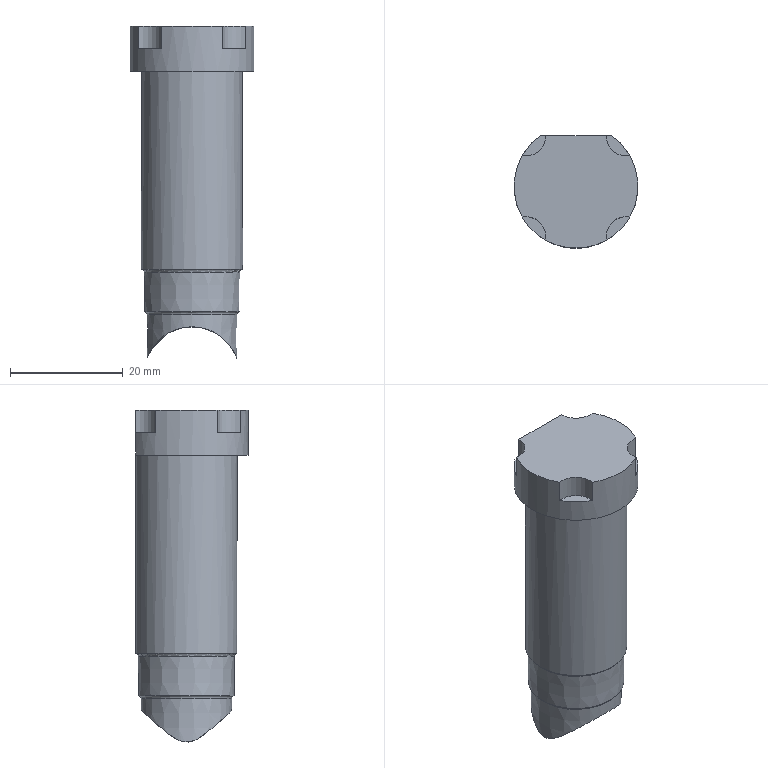Part | NX | features solid 2 | 1 solid | 18 faces | box 22 x 20 x 58.945 mm | volume 14202 mm3 | plane 7 | cylinder 6 | cone 3 | torus 2 | commonest cylinder face diameters 7 x4 18 x1 22 x1
STEP:
#1=CARTESIAN_POINT('',(9.556,23.036,66.5));
#2=VERTEX_POINT('',#1);
#3=CARTESIAN_POINT('',(6.325,26.587,66.5));
#4=VERTEX_POINT('',#3);
#5=CARTESIAN_POINT('',(0.,17.587,66.5));
#6=DIRECTION('',(0.,0.,-1.));
#7=DIRECTION('',(-1.,0.,0.));
#8=AXIS2_PLACEMENT_3D('',#5,#6,#7);
#9=CIRCLE('',#8,11.);
#10=EDGE_CURVE('',#2,#4,#9,.F.);
#11=ORIENTED_EDGE('',*,*,#10,.F.);
#12=CARTESIAN_POINT('',(9.556,23.036,70.5));
#13=VERTEX_POINT('',#12);
#14=CARTESIAN_POINT('',(9.556,23.036,66.5));
#15=DIRECTION('',(0.,0.,-1.));
#16=VECTOR('',#15,1000.);
#17=LINE('',#14,#16);
#18=EDGE_CURVE('',#2,#13,#17,.F.);
#19=ORIENTED_EDGE('',*,*,#18,.T.);
#20=CARTESIAN_POINT('',(9.556,12.139,70.5));
#21=VERTEX_POINT('',#20);
#22=CARTESIAN_POINT('',(0.,17.587,70.5));
#23=DIRECTION('',(0.,0.,1.));
#24=DIRECTION('',(1.,0.,0.));
#25=AXIS2_PLACEMENT_3D('',#22,#23,#24);
#26=CIRCLE('',#25,11.);
#27=EDGE_CURVE('',#21,#13,#26,.T.);
#28=ORIENTED_EDGE('',*,*,#27,.F.);
#29=CARTESIAN_POINT('',(9.556,12.139,66.5));
#30=VERTEX_POINT('',#29);
#31=CARTESIAN_POINT('',(9.556,12.139,66.5));
#32=DIRECTION('',(0.,0.,1.));
#33=VECTOR('',#32,1000.);
#34=LINE('',#31,#33);
#35=EDGE_CURVE('',#21,#30,#34,.F.);
#36=ORIENTED_EDGE('',*,*,#35,.T.);
#37=CARTESIAN_POINT('',(5.448,8.032,66.5));
#38=VERTEX_POINT('',#37);
#39=CARTESIAN_POINT('',(0.,17.587,66.5));
#40=DIRECTION('',(0.,0.,-1.));
#41=DIRECTION('',(-1.,0.,0.));
#42=AXIS2_PLACEMENT_3D('',#39,#40,#41);
#43=CIRCLE('',#42,11.);
#44=EDGE_CURVE('',#38,#30,#43,.F.);
#45=ORIENTED_EDGE('',*,*,#44,.F.);
#46=CARTESIAN_POINT('',(5.448,8.032,70.5));
#47=VERTEX_POINT('',#46);
#48=CARTESIAN_POINT('',(5.448,8.032,66.5));
#49=DIRECTION('',(0.,0.,1.));
#50=VECTOR('',#49,1000.);
#51=LINE('',#48,#50);
#52=EDGE_CURVE('',#38,#47,#51,.T.);
#53=ORIENTED_EDGE('',*,*,#52,.T.);
#54=CARTESIAN_POINT('',(-5.448,8.032,70.5));
#55=VERTEX_POINT('',#54);
#56=CARTESIAN_POINT('',(0.,17.587,70.5));
#57=DIRECTION('',(0.,0.,1.));
#58=DIRECTION('',(1.,0.,0.));
#59=AXIS2_PLACEMENT_3D('',#56,#57,#58);
#60=CIRCLE('',#59,11.);
#61=EDGE_CURVE('',#55,#47,#60,.T.);
#62=ORIENTED_EDGE('',*,*,#61,.F.);
#63=CARTESIAN_POINT('',(-5.448,8.032,66.5));
#64=VERTEX_POINT('',#63);
#65=CARTESIAN_POINT('',(-5.448,8.032,66.5));
#66=DIRECTION('',(0.,0.,1.));
#67=VECTOR('',#66,1000.);
#68=LINE('',#65,#67);
#69=EDGE_CURVE('',#55,#64,#68,.F.);
#70=ORIENTED_EDGE('',*,*,#69,.T.);
#71=CARTESIAN_POINT('',(-9.556,12.139,66.5));
#72=VERTEX_POINT('',#71);
#73=CARTESIAN_POINT('',(0.,17.587,66.5));
#74=DIRECTION('',(0.,0.,-1.));
#75=DIRECTION('',(-1.,0.,0.));
#76=AXIS2_PLACEMENT_3D('',#73,#74,#75);
#77=CIRCLE('',#76,11.);
#78=EDGE_CURVE('',#72,#64,#77,.F.);
#79=ORIENTED_EDGE('',*,*,#78,.F.);
#80=CARTESIAN_POINT('',(-9.556,12.139,70.5));
#81=VERTEX_POINT('',#80);
#82=CARTESIAN_POINT('',(-9.556,12.139,66.5));
#83=DIRECTION('',(0.,0.,1.));
#84=VECTOR('',#83,1000.);
#85=LINE('',#82,#84);
#86=EDGE_CURVE('',#72,#81,#85,.T.);
#87=ORIENTED_EDGE('',*,*,#86,.T.);
#88=CARTESIAN_POINT('',(-9.556,23.036,70.5));
#89=VERTEX_POINT('',#88);
#90=CARTESIAN_POINT('',(0.,17.587,70.5));
#91=DIRECTION('',(0.,0.,1.));
#92=DIRECTION('',(1.,0.,0.));
#93=AXIS2_PLACEMENT_3D('',#90,#91,#92);
#94=CIRCLE('',#93,11.);
#95=EDGE_CURVE('',#89,#81,#94,.T.);
#96=ORIENTED_EDGE('',*,*,#95,.F.);
#97=CARTESIAN_POINT('',(-9.556,23.036,66.5));
#98=VERTEX_POINT('',#97);
#99=CARTESIAN_POINT('',(-9.556,23.036,66.5));
#100=DIRECTION('',(0.,0.,1.));
#101=VECTOR('',#100,1000.);
#102=LINE('',#99,#101);
#103=EDGE_CURVE('',#89,#98,#102,.F.);
#104=ORIENTED_EDGE('',*,*,#103,.T.);
#105=CARTESIAN_POINT('',(-6.325,26.587,66.5));
#106=VERTEX_POINT('',#105);
#107=CARTESIAN_POINT('',(0.,17.587,66.5));
#108=DIRECTION('',(0.,0.,-1.));
#109=DIRECTION('',(-1.,0.,0.));
#110=AXIS2_PLACEMENT_3D('',#107,#108,#109);
#111=CIRCLE('',#110,11.);
#112=EDGE_CURVE('',#106,#98,#111,.F.);
#113=ORIENTED_EDGE('',*,*,#112,.F.);
#114=CARTESIAN_POINT('',(-6.325,26.587,62.5));
#115=VERTEX_POINT('',#114);
#116=CARTESIAN_POINT('',(-6.325,26.587,62.5));
#117=DIRECTION('',(0.,0.,1.));
#118=VECTOR('',#117,1000.);
#119=LINE('',#116,#118);
#120=EDGE_CURVE('',#106,#115,#119,.F.);
#121=ORIENTED_EDGE('',*,*,#120,.T.);
#122=CARTESIAN_POINT('',(6.325,26.587,62.5));
#123=VERTEX_POINT('',#122);
#124=CARTESIAN_POINT('',(0.,17.587,62.5));
#125=DIRECTION('',(0.,0.,1.));
#126=DIRECTION('',(1.,0.,0.));
#127=AXIS2_PLACEMENT_3D('',#124,#125,#126);
#128=CIRCLE('',#127,11.);
#129=EDGE_CURVE('',#115,#123,#128,.T.);
#130=ORIENTED_EDGE('',*,*,#129,.T.);
#131=CARTESIAN_POINT('',(6.325,26.587,62.5));
#132=DIRECTION('',(0.,0.,1.));
#133=VECTOR('',#132,1000.);
#134=LINE('',#131,#133);
#135=EDGE_CURVE('',#123,#4,#134,.T.);
#136=ORIENTED_EDGE('',*,*,#135,.T.);
#137=EDGE_LOOP('',(#11,#19,#28,#36,#45,#53,#62,#70,#79,#87,#96,#104,#113,#121,#130,#136));
#138=FACE_BOUND('',#137,.T.);
#139=CARTESIAN_POINT('',(0.,17.587,62.5));
#140=DIRECTION('',(0.,0.,1.));
#141=DIRECTION('',(1.,0.,0.));
#142=AXIS2_PLACEMENT_3D('',#139,#140,#141);
#143=CYLINDRICAL_SURFACE('',#142,11.);
#144=ADVANCED_FACE('',(#138),#143,.T.);
#145=ORIENTED_EDGE('',*,*,#27,.T.);
#146=CARTESIAN_POINT('',(5.385,26.587,70.5));
#147=VERTEX_POINT('',#146);
#148=CARTESIAN_POINT('',(8.883,26.471,70.5));
#149=DIRECTION('',(0.,0.,1.));
#150=DIRECTION('',(1.,0.,0.));
#151=AXIS2_PLACEMENT_3D('',#148,#149,#150);
#152=CIRCLE('',#151,3.5);
#153=EDGE_CURVE('',#13,#147,#152,.F.);
#154=ORIENTED_EDGE('',*,*,#153,.T.);
#155=CARTESIAN_POINT('',(-5.385,26.587,70.5));
#156=VERTEX_POINT('',#155);
#157=CARTESIAN_POINT('',(0.,26.587,70.5));
#158=DIRECTION('',(-1.,0.,0.));
#159=VECTOR('',#158,1000.);
#160=LINE('',#157,#159);
#161=EDGE_CURVE('',#147,#156,#160,.T.);
#162=ORIENTED_EDGE('',*,*,#161,.T.);
#163=CARTESIAN_POINT('',(-8.883,26.471,70.5));
#164=DIRECTION('',(0.,0.,1.));
#165=DIRECTION('',(1.,0.,0.));
#166=AXIS2_PLACEMENT_3D('',#163,#164,#165);
#167=CIRCLE('',#166,3.5);
#168=EDGE_CURVE('',#156,#89,#167,.F.);
#169=ORIENTED_EDGE('',*,*,#168,.T.);
#170=ORIENTED_EDGE('',*,*,#95,.T.);
#171=CARTESIAN_POINT('',(-8.883,8.704,70.5));
#172=DIRECTION('',(0.,0.,1.));
#173=DIRECTION('',(1.,0.,0.));
#174=AXIS2_PLACEMENT_3D('',#171,#172,#173);
#175=CIRCLE('',#174,3.5);
#176=EDGE_CURVE('',#81,#55,#175,.F.);
#177=ORIENTED_EDGE('',*,*,#176,.T.);
#178=ORIENTED_EDGE('',*,*,#61,.T.);
#179=CARTESIAN_POINT('',(8.883,8.704,70.5));
#180=DIRECTION('',(0.,0.,1.));
#181=DIRECTION('',(1.,0.,0.));
#182=AXIS2_PLACEMENT_3D('',#179,#180,#181);
#183=CIRCLE('',#182,3.5);
#184=EDGE_CURVE('',#47,#21,#183,.F.);
#185=ORIENTED_EDGE('',*,*,#184,.T.);
#186=EDGE_LOOP('',(#145,#154,#162,#169,#170,#177,#178,#185));
#187=FACE_BOUND('',#186,.T.);
#188=CARTESIAN_POINT('',(0.,0.,70.5));
#189=DIRECTION('',(0.,0.,1.));
#190=DIRECTION('',(1.,0.,0.));
#191=AXIS2_PLACEMENT_3D('',#188,#189,#190);
#192=PLANE('',#191);
#193=ADVANCED_FACE('',(#187),#192,.T.);
#194=ORIENTED_EDGE('',*,*,#161,.F.);
#195=CARTESIAN_POINT('',(5.385,26.587,66.5));
#196=VERTEX_POINT('',#195);
#197=CARTESIAN_POINT('',(5.385,26.587,70.5));
#198=DIRECTION('',(0.,0.,1.));
#199=VECTOR('',#198,1000.);
#200=LINE('',#197,#199);
#201=EDGE_CURVE('',#147,#196,#200,.F.);
#202=ORIENTED_EDGE('',*,*,#201,.T.);
#203=CARTESIAN_POINT('',(0.,26.587,66.5));
#204=DIRECTION('',(-1.,0.,0.));
#205=VECTOR('',#204,1000.);
#206=LINE('',#203,#205);
#207=EDGE_CURVE('',#4,#196,#206,.T.);
#208=ORIENTED_EDGE('',*,*,#207,.F.);
#209=ORIENTED_EDGE('',*,*,#135,.F.);
#210=CARTESIAN_POINT('',(0.,26.587,62.5));
#211=VERTEX_POINT('',#210);
#212=CARTESIAN_POINT('',(0.,26.587,62.5));
#213=DIRECTION('',(-1.,0.,0.));
#214=VECTOR('',#213,1000.);
#215=LINE('',#212,#214);
#216=EDGE_CURVE('',#123,#211,#215,.T.);
#217=ORIENTED_EDGE('',*,*,#216,.T.);
#218=CARTESIAN_POINT('',(0.,26.587,62.5));
#219=DIRECTION('',(-1.,0.,0.));
#220=VECTOR('',#219,1000.);
#221=LINE('',#218,#220);
#222=EDGE_CURVE('',#211,#115,#221,.T.);
#223=ORIENTED_EDGE('',*,*,#222,.T.);
#224=ORIENTED_EDGE('',*,*,#120,.F.);
#225=CARTESIAN_POINT('',(-5.385,26.587,66.5));
#226=VERTEX_POINT('',#225);
#227=CARTESIAN_POINT('',(0.,26.587,66.5));
#228=DIRECTION('',(-1.,0.,0.));
#229=VECTOR('',#228,1000.);
#230=LINE('',#227,#229);
#231=EDGE_CURVE('',#226,#106,#230,.T.);
#232=ORIENTED_EDGE('',*,*,#231,.F.);
#233=CARTESIAN_POINT('',(-5.385,26.587,66.5));
#234=DIRECTION('',(0.,0.,1.));
#235=VECTOR('',#234,1000.);
#236=LINE('',#233,#235);
#237=EDGE_CURVE('',#226,#156,#236,.T.);
#238=ORIENTED_EDGE('',*,*,#237,.T.);
#239=EDGE_LOOP('',(#194,#202,#208,#209,#217,#223,#224,#232,#238));
#240=FACE_BOUND('',#239,.T.);
#241=CARTESIAN_POINT('',(0.,26.587,62.5));
#242=DIRECTION('',(0.,1.,0.));
#243=DIRECTION('',(0.,0.,1.));
#244=AXIS2_PLACEMENT_3D('',#241,#242,#243);
#245=PLANE('',#244);
#246=ADVANCED_FACE('',(#240),#245,.T.);
#247=ORIENTED_EDGE('',*,*,#216,.F.);
#248=ORIENTED_EDGE('',*,*,#129,.F.);
#249=ORIENTED_EDGE('',*,*,#222,.F.);
#250=CARTESIAN_POINT('',(0.,17.587,62.5));
#251=DIRECTION('',(0.,0.,1.));
#252=DIRECTION('',(1.,0.,0.));
#253=AXIS2_PLACEMENT_3D('',#250,#251,#252);
#254=CIRCLE('',#253,9.);
#255=EDGE_CURVE('',#211,#211,#254,.T.);
#256=ORIENTED_EDGE('',*,*,#255,.T.);
#257=EDGE_LOOP('',(#247,#248,#249,#256));
#258=FACE_BOUND('',#257,.T.);
#259=CARTESIAN_POINT('',(0.,17.587,62.5));
#260=DIRECTION('',(0.,0.,1.));
#261=DIRECTION('',(1.,0.,0.));
#262=AXIS2_PLACEMENT_3D('',#259,#260,#261);
#263=PLANE('',#262);
#264=ADVANCED_FACE('',(#258),#263,.F.);
#265=ORIENTED_EDGE('',*,*,#255,.F.);
#266=EDGE_LOOP('',(#265));
#267=FACE_BOUND('',#266,.T.);
#268=CARTESIAN_POINT('',(-9.,17.587,27.316));
#269=VERTEX_POINT('',#268);
#270=CARTESIAN_POINT('',(0.,17.587,27.316));
#271=DIRECTION('',(0.,0.,-1.));
#272=DIRECTION('',(-1.,0.,0.));
#273=AXIS2_PLACEMENT_3D('',#270,#271,#272);
#274=CIRCLE('',#273,9.);
#275=EDGE_CURVE('',#269,#269,#274,.T.);
#276=ORIENTED_EDGE('',*,*,#275,.F.);
#277=EDGE_LOOP('',(#276));
#278=FACE_BOUND('',#277,.T.);
#279=CARTESIAN_POINT('',(0.,17.587,-72.682));
#280=DIRECTION('',(0.,0.,1.));
#281=DIRECTION('',(1.,0.,0.));
#282=AXIS2_PLACEMENT_3D('',#279,#280,#281);
#283=CYLINDRICAL_SURFACE('',#282,9.);
#284=ADVANCED_FACE('',(#267,#278),#283,.T.);
#285=CARTESIAN_POINT('',(-5.996,12.299,14.621));
#286=VERTEX_POINT('',#285);
#287=CARTESIAN_POINT('',(-3.768,10.267,16.455));
#288=CARTESIAN_POINT('',(-5.753,11.888,14.966));
#289=CARTESIAN_POINT('',(-6.878,13.445,13.632));
#290=CARTESIAN_POINT('',(-7.493,14.728,12.644));
#291=CARTESIAN_POINT('',(-7.907,16.191,11.711));
#292=CARTESIAN_POINT('',(-8.023,17.994,11.407));
#293=CARTESIAN_POINT('',(-7.76,19.619,12.176));
#294=CARTESIAN_POINT('',(-7.271,20.98,13.149));
#295=CARTESIAN_POINT('',(-6.565,22.218,14.168));
#296=CARTESIAN_POINT('',(-5.326,23.697,15.471));
#297=CARTESIAN_POINT('',(-3.18,25.199,16.865));
#298=CARTESIAN_POINT('',(0.3652,25.87,17.5));
#299=CARTESIAN_POINT('',(3.775,24.908,16.591));
#300=CARTESIAN_POINT('',(6.159,22.95,14.791));
#301=CARTESIAN_POINT('',(7.357,20.926,13.065));
#302=CARTESIAN_POINT('',(7.901,19.005,11.8));
#303=CARTESIAN_POINT('',(8.025,17.233,11.377));
#304=CARTESIAN_POINT('',(7.765,15.57,12.072));
#305=CARTESIAN_POINT('',(7.108,13.745,13.353));
#306=CARTESIAN_POINT('',(5.755,11.779,15.061));
#307=CARTESIAN_POINT('',(3.17,9.974,16.728));
#308=CARTESIAN_POINT('',(-0.3609,9.307,17.359));
#309=CARTESIAN_POINT('',(-3.768,10.267,16.455));
#310=CARTESIAN_POINT('',(-5.753,11.888,14.966));
#311=CARTESIAN_POINT('',(-6.878,13.445,13.632));
#312=B_SPLINE_CURVE_WITH_KNOTS('',3,(#287,#288,#289,#290,#291,#292,#293,#294,#295,#296,#297,#298,#299,#300,#301,#302,#303,#304,#305,#306,#307,#308,#309,#310,#311),.UNSPECIFIED.,.T.,.F.,(1,1,1,1,1,1,1,1,1,1,1,1,1,1,1,1,1,1,1,1,1,1,1,1,1,1,1,1,1),(-0.01042,-0.006944,-0.003472,0.,0.001736,0.003472,0.005208,0.006944,0.00868,0.01042,0.01215,0.01389,0.01736,0.02083,0.0243,0.02778,0.03125,0.03298,0.03472,0.03646,0.03819,0.04166,0.04514,0.04861,0.05208,0.05555,0.05729,0.05902,0.06076),.UNSPECIFIED.);
#313=EDGE_CURVE('',#286,#286,#312,.T.);
#314=ORIENTED_EDGE('',*,*,#313,.T.);
#315=EDGE_LOOP('',(#314));
#316=FACE_BOUND('',#315,.T.);
#317=CARTESIAN_POINT('',(0.,14.447,8.725));
#318=DIRECTION('',(0.,1.,0.));
#319=DIRECTION('',(0.,0.,-1.));
#320=AXIS2_PLACEMENT_3D('',#317,#318,#319);
#321=CONICAL_SURFACE('',#320,8.427,0.008727);
#322=ADVANCED_FACE('',(#316),#321,.F.);
#323=ORIENTED_EDGE('',*,*,#313,.F.);
#324=EDGE_LOOP('',(#323));
#325=FACE_BOUND('',#324,.T.);
#326=CARTESIAN_POINT('',(0.,9.552,19.286));
#327=VERTEX_POINT('',#326);
#328=CARTESIAN_POINT('',(0.,17.587,19.286));
#329=DIRECTION('',(0.,0.,1.));
#330=DIRECTION('',(0.,-1.,0.));
#331=AXIS2_PLACEMENT_3D('',#328,#329,#330);
#332=CIRCLE('',#331,8.036);
#333=EDGE_CURVE('',#327,#327,#332,.F.);
#334=ORIENTED_EDGE('',*,*,#333,.T.);
#335=EDGE_LOOP('',(#334));
#336=FACE_BOUND('',#335,.T.);
#337=CARTESIAN_POINT('',(0.,17.587,15.418));
#338=DIRECTION('',(0.,0.,1.));
#339=DIRECTION('',(0.,-1.,0.));
#340=AXIS2_PLACEMENT_3D('',#337,#338,#339);
#341=CONICAL_SURFACE('',#340,8.002,0.008727);
#342=ADVANCED_FACE('',(#325,#336),#341,.T.);
#343=CARTESIAN_POINT('',(0.,9.111,19.78));
#344=VERTEX_POINT('',#343);
#345=CARTESIAN_POINT('',(0.,17.587,19.78));
#346=DIRECTION('',(0.,0.,1.));
#347=DIRECTION('',(0.,-1.,0.));
#348=AXIS2_PLACEMENT_3D('',#345,#346,#347);
#349=CIRCLE('',#348,8.477);
#350=EDGE_CURVE('',#344,#344,#349,.F.);
#351=ORIENTED_EDGE('',*,*,#350,.T.);
#352=EDGE_LOOP('',(#351));
#353=FACE_BOUND('',#352,.T.);
#354=ORIENTED_EDGE('',*,*,#333,.F.);
#355=EDGE_LOOP('',(#354));
#356=FACE_BOUND('',#355,.T.);
#357=CARTESIAN_POINT('',(0.,17.587,19.281));
#358=DIRECTION('',(0.,0.,1.));
#359=DIRECTION('',(0.0004539,1.,0.));
#360=AXIS2_PLACEMENT_3D('',#357,#358,#359);
#361=TOROIDAL_SURFACE('',#360,8.538,0.5025);
#362=ADVANCED_FACE('',(#353,#356),#361,.F.);
#363=CARTESIAN_POINT('',(0.,9.049,26.82));
#364=VERTEX_POINT('',#363);
#365=CARTESIAN_POINT('',(0.,17.587,26.82));
#366=DIRECTION('',(0.,0.,1.));
#367=DIRECTION('',(0.,-1.,0.));
#368=AXIS2_PLACEMENT_3D('',#365,#366,#367);
#369=CIRCLE('',#368,8.538);
#370=EDGE_CURVE('',#364,#364,#369,.F.);
#371=ORIENTED_EDGE('',*,*,#370,.T.);
#372=EDGE_LOOP('',(#371));
#373=FACE_BOUND('',#372,.T.);
#374=ORIENTED_EDGE('',*,*,#350,.F.);
#375=EDGE_LOOP('',(#374));
#376=FACE_BOUND('',#375,.T.);
#377=CARTESIAN_POINT('',(0.,17.587,23.3));
#378=DIRECTION('',(0.,0.,1.));
#379=DIRECTION('',(0.,-1.,0.));
#380=AXIS2_PLACEMENT_3D('',#377,#378,#379);
#381=CONICAL_SURFACE('',#380,8.507,0.008727);
#382=ADVANCED_FACE('',(#373,#376),#381,.T.);
#383=ORIENTED_EDGE('',*,*,#275,.T.);
#384=EDGE_LOOP('',(#383));
#385=FACE_BOUND('',#384,.T.);
#386=ORIENTED_EDGE('',*,*,#370,.F.);
#387=EDGE_LOOP('',(#386));
#388=FACE_BOUND('',#387,.T.);
#389=CARTESIAN_POINT('',(0.,17.587,26.815));
#390=DIRECTION('',(0.,0.,1.));
#391=DIRECTION('',(0.03571,0.9994,0.));
#392=AXIS2_PLACEMENT_3D('',#389,#390,#391);
#393=TOROIDAL_SURFACE('',#392,9.041,0.5025);
#394=ADVANCED_FACE('',(#385,#388),#393,.F.);
#395=ORIENTED_EDGE('',*,*,#168,.F.);
#396=ORIENTED_EDGE('',*,*,#237,.F.);
#397=CARTESIAN_POINT('',(-8.883,26.471,66.5));
#398=DIRECTION('',(0.,0.,-1.));
#399=DIRECTION('',(-1.,0.,0.));
#400=AXIS2_PLACEMENT_3D('',#397,#398,#399);
#401=CIRCLE('',#400,3.5);
#402=EDGE_CURVE('',#98,#226,#401,.F.);
#403=ORIENTED_EDGE('',*,*,#402,.F.);
#404=ORIENTED_EDGE('',*,*,#103,.F.);
#405=EDGE_LOOP('',(#395,#396,#403,#404));
#406=FACE_BOUND('',#405,.T.);
#407=CARTESIAN_POINT('',(-8.883,26.471,66.5));
#408=DIRECTION('',(0.,0.,1.));
#409=DIRECTION('',(1.,0.,0.));
#410=AXIS2_PLACEMENT_3D('',#407,#408,#409);
#411=CYLINDRICAL_SURFACE('',#410,3.5);
#412=ADVANCED_FACE('',(#406),#411,.F.);
#413=ORIENTED_EDGE('',*,*,#112,.T.);
#414=ORIENTED_EDGE('',*,*,#402,.T.);
#415=ORIENTED_EDGE('',*,*,#231,.T.);
#416=EDGE_LOOP('',(#413,#414,#415));
#417=FACE_BOUND('',#416,.T.);
#418=CARTESIAN_POINT('',(-8.883,26.471,66.5));
#419=DIRECTION('',(0.,0.,-1.));
#420=DIRECTION('',(-1.,0.,0.));
#421=AXIS2_PLACEMENT_3D('',#418,#419,#420);
#422=PLANE('',#421);
#423=ADVANCED_FACE('',(#417),#422,.F.);
#424=ORIENTED_EDGE('',*,*,#176,.F.);
#425=ORIENTED_EDGE('',*,*,#86,.F.);
#426=CARTESIAN_POINT('',(-8.883,8.704,66.5));
#427=DIRECTION('',(0.,0.,-1.));
#428=DIRECTION('',(-1.,0.,0.));
#429=AXIS2_PLACEMENT_3D('',#426,#427,#428);
#430=CIRCLE('',#429,3.5);
#431=EDGE_CURVE('',#64,#72,#430,.F.);
#432=ORIENTED_EDGE('',*,*,#431,.F.);
#433=ORIENTED_EDGE('',*,*,#69,.F.);
#434=EDGE_LOOP('',(#424,#425,#432,#433));
#435=FACE_BOUND('',#434,.T.);
#436=CARTESIAN_POINT('',(-8.883,8.704,66.5));
#437=DIRECTION('',(0.,0.,1.));
#438=DIRECTION('',(1.,0.,0.));
#439=AXIS2_PLACEMENT_3D('',#436,#437,#438);
#440=CYLINDRICAL_SURFACE('',#439,3.5);
#441=ADVANCED_FACE('',(#435),#440,.F.);
#442=ORIENTED_EDGE('',*,*,#78,.T.);
#443=ORIENTED_EDGE('',*,*,#431,.T.);
#444=EDGE_LOOP('',(#442,#443));
#445=FACE_BOUND('',#444,.T.);
#446=CARTESIAN_POINT('',(-8.883,8.704,66.5));
#447=DIRECTION('',(0.,0.,-1.));
#448=DIRECTION('',(-1.,0.,0.));
#449=AXIS2_PLACEMENT_3D('',#446,#447,#448);
#450=PLANE('',#449);
#451=ADVANCED_FACE('',(#445),#450,.F.);
#452=ORIENTED_EDGE('',*,*,#184,.F.);
#453=ORIENTED_EDGE('',*,*,#52,.F.);
#454=CARTESIAN_POINT('',(8.883,8.704,66.5));
#455=DIRECTION('',(0.,0.,-1.));
#456=DIRECTION('',(-1.,0.,0.));
#457=AXIS2_PLACEMENT_3D('',#454,#455,#456);
#458=CIRCLE('',#457,3.5);
#459=EDGE_CURVE('',#30,#38,#458,.F.);
#460=ORIENTED_EDGE('',*,*,#459,.F.);
#461=ORIENTED_EDGE('',*,*,#35,.F.);
#462=EDGE_LOOP('',(#452,#453,#460,#461));
#463=FACE_BOUND('',#462,.T.);
#464=CARTESIAN_POINT('',(8.883,8.704,66.5));
#465=DIRECTION('',(0.,0.,1.));
#466=DIRECTION('',(1.,0.,0.));
#467=AXIS2_PLACEMENT_3D('',#464,#465,#466);
#468=CYLINDRICAL_SURFACE('',#467,3.5);
#469=ADVANCED_FACE('',(#463),#468,.F.);
#470=ORIENTED_EDGE('',*,*,#44,.T.);
#471=ORIENTED_EDGE('',*,*,#459,.T.);
#472=EDGE_LOOP('',(#470,#471));
#473=FACE_BOUND('',#472,.T.);
#474=CARTESIAN_POINT('',(8.883,8.704,66.5));
#475=DIRECTION('',(0.,0.,-1.));
#476=DIRECTION('',(-1.,0.,0.));
#477=AXIS2_PLACEMENT_3D('',#474,#475,#476);
#478=PLANE('',#477);
#479=ADVANCED_FACE('',(#473),#478,.F.);
#480=CARTESIAN_POINT('',(8.883,26.471,66.5));
#481=DIRECTION('',(0.,0.,-1.));
#482=DIRECTION('',(-1.,0.,0.));
#483=AXIS2_PLACEMENT_3D('',#480,#481,#482);
#484=CIRCLE('',#483,3.5);
#485=EDGE_CURVE('',#196,#2,#484,.F.);
#486=ORIENTED_EDGE('',*,*,#485,.F.);
#487=ORIENTED_EDGE('',*,*,#201,.F.);
#488=ORIENTED_EDGE('',*,*,#153,.F.);
#489=ORIENTED_EDGE('',*,*,#18,.F.);
#490=EDGE_LOOP('',(#486,#487,#488,#489));
#491=FACE_BOUND('',#490,.T.);
#492=CARTESIAN_POINT('',(8.883,26.471,66.5));
#493=DIRECTION('',(0.,0.,1.));
#494=DIRECTION('',(1.,0.,0.));
#495=AXIS2_PLACEMENT_3D('',#492,#493,#494);
#496=CYLINDRICAL_SURFACE('',#495,3.5);
#497=ADVANCED_FACE('',(#491),#496,.F.);
#498=ORIENTED_EDGE('',*,*,#10,.T.);
#499=ORIENTED_EDGE('',*,*,#207,.T.);
#500=ORIENTED_EDGE('',*,*,#485,.T.);
#501=EDGE_LOOP('',(#498,#499,#500));
#502=FACE_BOUND('',#501,.T.);
#503=CARTESIAN_POINT('',(8.883,26.471,66.5));
#504=DIRECTION('',(0.,0.,-1.));
#505=DIRECTION('',(-1.,0.,0.));
#506=AXIS2_PLACEMENT_3D('',#503,#504,#505);
#507=PLANE('',#506);
#508=ADVANCED_FACE('',(#502),#507,.F.);
#509=CLOSED_SHELL('',(#144,#193,#246,#264,#284,#322,#342,#362,#382,#394,#412,#423,#441,#451,#469,#479,#497,#508));
#510=MANIFOLD_SOLID_BREP('',#509);
#511=(LENGTH_UNIT()NAMED_UNIT(*)SI_UNIT(.MILLI.,.METRE.));
#512=UNCERTAINTY_MEASURE_WITH_UNIT(LENGTH_MEASURE(0.0508),#511,'','');
#513=(NAMED_UNIT(*)PLANE_ANGLE_UNIT()SI_UNIT($,.RADIAN.));
#514=(NAMED_UNIT(*)SI_UNIT($,.STERADIAN.)SOLID_ANGLE_UNIT());
#515=(GEOMETRIC_REPRESENTATION_CONTEXT(3)GLOBAL_UNCERTAINTY_ASSIGNED_CONTEXT((#512))GLOBAL_UNIT_ASSIGNED_CONTEXT((#511,#513,#514))REPRESENTATION_CONTEXT('',''));
#516=ADVANCED_BREP_SHAPE_REPRESENTATION('',(#510),#515);